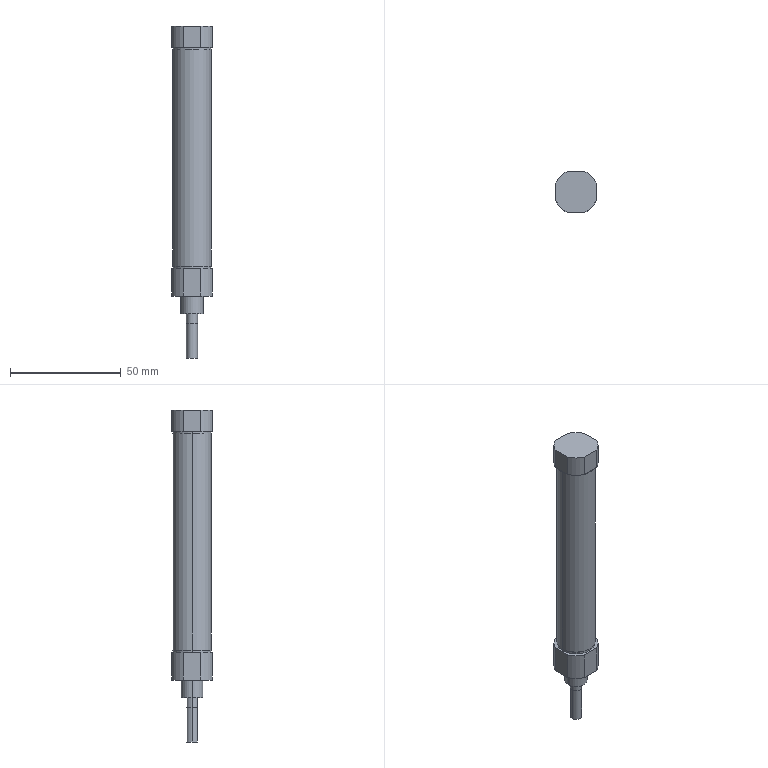Part | STEP file | CDJ2B16-75-B | 3 solids | 48 faces | box 18.4 x 18.4 x 150.2 mm | volume 31123 mm3 | cylinder 26 | plane 22 | commonest cylinder face diameters 20 x8 4 x4 5 x4 17 x4 5.2 x2 10 x2